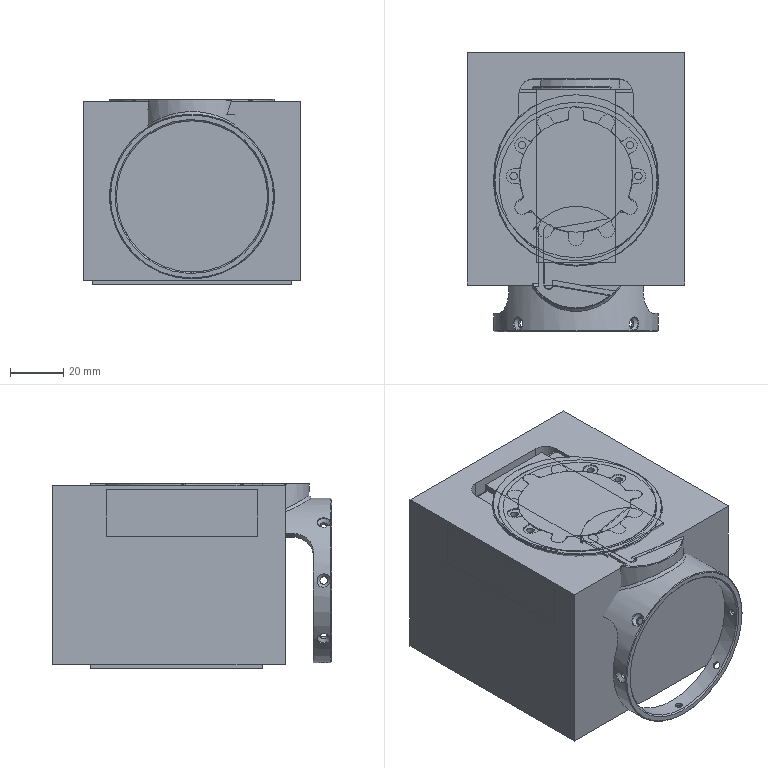NC program | NX | posted with a generic post | part box 82 x 105.2 x 70 mm
Lines 22992 to 23469 of 123648:
(单向轮廓精光_3_COPY_1_COPY_COPY_COPY_COPY , TOOL : 光刀D4)
N45862 T07 M6
N45864 G53
N45866 G18 G0 G90 X15.218 Z-47.555 S12000 M3
N45868 G43 Y73.855 H7
N45870 Y28.155
N45872 G41 G94 G1 Z-42.355 F700. D7
N45874 Z-40.63
N45876 G2 X13.549 Z-38.641 R2.02
N45878 G1 X-8.153 Z-34.814
N45880 G2 X-9.46 Z-35.024 R2.02
N45882 G1 X-9.622 Z-35.111
N45884 X-9.78 Z-35.206
N45886 Z-20.749
N45888 G2 X-9.573 Z-20.877 R2.02
N45890 G1 X-9.407 Z-20.966
N45892 G2 X-8.1 Z-21.176 R2.02
N45894 G1 X13.298 Z-17.403
N45896 G2 X14.29 Z-16.923 R2.02
N45898 G1 X14.407 Z-16.819
N45900 G2 X14.783 Z-16.371 R2.02
N45902 G1 X14.917 Z-16.153
N45904 G2 X15.218 Z-15.092 R2.02
N45906 G1 Z-13.645
N45908 Z-8.645
N45910 G40
N45912 Z-8.445
N45914 G0 Y73.855
N45916 X15.198 Z-47.555
N45918 Y28.155
N45920 G41 G1 Z-42.355
N45922 Z-40.63
N45924 G2 X13.545 Z-38.661 R2.
N45926 G1 X-8.157 Z-34.834
N45928 G2 X-9.451 Z-35.042 R2.
N45930 G1 X-9.613 Z-35.129
N45932 G2 X-9.8 Z-35.243 R2.
N45934 G1 Z-20.71
N45936 G2 X-9.563 Z-20.86 R2.
N45938 G1 X-9.398 Z-20.949
N45940 G2 X-8.104 Z-21.157 R2.
N45942 G1 X13.294 Z-17.384
N45944 G2 X14.277 Z-16.908 R2.
N45946 G1 X14.393 Z-16.804
N45948 G2 X14.766 Z-16.36 R2.
N45950 G1 X14.9 Z-16.142
N45952 G2 X15.198 Z-15.092 R2.
N45954 G1 Z-13.645
N45956 Z-8.645
N45958 G40
N45960 Z-8.445
N45962 G0 Y73.855
(单向轮廓精光_3_COPY_1_COPY_COPY_COPY , TOOL : 光刀D4)
N45964 X15.417 Z-37.258
N45966 Y73.84
N45968 Y33.14
N45970 G41 G1 X14.878 Z-40.311
N45972 G3 X14.531 Z-40.554 R0.3
N45974 G1 X-9.437 Z-36.328
N45976 G3 X-9.68 Z-35.98 R0.3
N45978 G1 X-9.176 Z-33.124
N45980 G40
N45982 X-9.142 Z-32.927
N45984 X15.417 Z-37.258
N45986 G41 X14.875 Z-40.33
N45988 G3 X14.527 Z-40.574 R0.3
N45990 G1 X-9.44 Z-36.348
N45992 G3 X-9.684 Z-36. R0.3
N45994 G1 X-9.176 Z-33.124
N45996 G40
N45998 X-9.142 Z-32.927
N46000 G0 Y73.84
N46002 Z-23.073
N46004 Y33.14
N46006 G41 G1 X-9.68 Z-20.02
N46008 G3 X-9.437 Z-19.672 R0.3
N46010 G1 X14.531 Z-15.446
N46012 G3 X14.878 Z-15.689 R0.3
N46014 G1 X15.382 Z-18.545
N46016 G40
N46018 X15.417 Z-18.742
N46020 X-9.142 Z-23.073
N46022 G41 X-9.683 Z-20.
N46024 G3 X-9.44 Z-19.652 R0.3
N46026 G1 X14.527 Z-15.426
N46028 G3 X14.875 Z-15.67 R0.3
N46030 G1 X15.382 Z-18.545
N46032 G40
N46034 X15.417 Z-18.742
N46036 G0 Y73.84
(底壁铣选底 , TOOL : 光刀D4)
N46038 Y77.5 S8000
N46040 X21.88 Z-30.292
N46042 Y29.15
N46044 G1 Y28.15 F1200.
N46046 X21.363 Z-30.874
N46048 G3 X20.798 Z-30.907 R0.4
N46050 G2 X15.681 Z-28.426 R10.4
N46052 G1 X13.264 Z-28.
N46054 X10.783
N46056 X13.264
N46058 X15.681 Z-27.574
N46060 G2 X20.798 Z-25.093 R10.4
N46062 X20.174 Z-22.168 R21.
N46064 G1 X19.061 Z-23.158
N46066 G3 X15.23 Z-25.013 R7.8
N46068 G1 X-1.708 Z-28.
N46070 X15.23 Z-30.987
N46072 G3 X19.061 Z-32.842 R7.8
N46074 G1 X20.174 Z-33.832
N46076 G3 X19.116 Z-36.693 R21.
N46078 G1 X18.677 Z-35.98
N46080 X17.333 Z-34.784
N46082 G2 X14.779 Z-33.547 R5.2
N46084 G1 X-4.55 Z-30.139
N46086 Z-25.861
N46088 X14.779 Z-22.453
N46090 G2 X17.333 Z-21.216 R5.2
N46092 G1 X18.677 Z-20.02
N46094 X19.116 Z-19.307
N46096 G2 X17.662 Z-16.64 R21.
N46098 G3 X17.461 Z-17.039 R2.6
N46100 G1 X16.664 Z-18.331
N46102 X15.604 Z-19.274
N46104 G3 X14.327 Z-19.892 R2.6
N46106 G1 X-7.15 Z-23.679
N46108 Z-32.321
N46110 X14.327 Z-36.108
N46112 G3 X15.604 Z-36.726 R2.6
N46114 G1 X16.664 Z-37.669
N46116 X17.461 Z-38.961
N46118 G3 X17.662 Z-39.36 R2.6
N46120 X15.401 Z-42.276 R21.
N46122 X15.248 Z-42.439 R21.
N46124 G1 Z-40.326
N46126 X14.651 Z-39.358
N46128 X13.876 Z-38.668
N46130 X-8.848 Z-34.661
N46132 X-9.636 Z-35.085
N46134 X-9.75 Z-35.151
N46136 Z-20.806
N46138 X-9.675 Z-20.857
N46140 X-9.587 Z-20.904
N46142 X-8.795 Z-21.329
N46144 X13.876 Z-17.332
N46146 X14.651 Z-16.642
N46148 X15.248 Z-15.674
N46150 Z-13.56
N46152 G3 X15.648 Z-13.16 R0.4
N46154 G1 X16.248
N46156 Y29.15
N46158 G0 Y77.5
N46160 M5
(单向轮廓精光_4 , TOOL : D10加长刀)
N46162 T10 M6
N46164 G53
N46166 G17 G0 G90 X25.02 Y43.85 S4500 M3
N46168 G43 Z40. H10
N46170 Z-56.5
N46172 G94 G1 Z-59.5 F700.
N46174 G41 Y35.65 D10
N46176 Y23.889
N46178 G3 X25.593 Y22.496 R1.98
N46180 G2 X-25.593 Y22.496 R-36.02
N46182 G3 X-25.02 Y23.889 R1.98
N46184 G1 Y35.65
N46186 Y43.65
N46188 G40
N46190 Y43.85
N46192 Z-56.5
N46194 G0 Z40.
N46196 X25.
N46198 Z-56.5
N46200 G1 Z-59.5
N46202 G41 Y35.65
N46204 Y23.889
N46206 G3 X25.579 Y22.482 R2.
N46208 G2 X-25.579 Y22.482 R-36.
N46210 G3 X-25. Y23.889 R2.
N46212 G1 Y35.65
N46214 Y43.65
N46216 G40
N46218 Y43.85
N46220 Z-56.5
N46222 G0 Z40.
N46224 X25.
N46226 Z-56.5
N46228 G1 Z-59.5
N46230 G41 Y35.65
N46232 Y23.889
N46234 G3 X25.579 Y22.482 R2.
N46236 G2 X-25.579 Y22.482 R-36.
N46238 G3 X-25. Y23.889 R2.
N46240 G1 Y35.65
N46242 Y43.65
N46244 G40
N46246 Y43.85
N46248 Z-56.5
N46250 G0 Z40.
N46252 X25.
N46254 Z-56.5
N46256 G1 Z-59.5
N46258 G41 Y35.65
N46260 Y23.889
N46262 G3 X25.579 Y22.482 R2.
N46264 G2 X-25.579 Y22.482 R-36.
N46266 G3 X-25. Y23.889 R2.
N46268 G1 Y35.65
N46270 Y43.65
N46272 G40
N46274 Y43.85
N46276 Z-56.5
N46278 G0 Z40.
N46280 M5
(单向轮廓精光_5 , TOOL : 光刀D8)
N46282 T08 M6
N46284 G53
N46286 G18 G0 G90 X1. Z-30.205 S8000 M3
N46288 G43 Y73.85 H8
N46290 Y23.15
N46292 G94 G1 Y20.15 F1200.
N46294 G41 Z-32.005 D8
N46296 G3 X0. Z-33.005 R1.
N46298 X-5.005 Z-28. R5.005
N46300 X0. Z-33.005 R-5.005
N46302 X-0.499 Z-32.98 R5.005
N46304 X-1.394 Z-31.885 R1.
N46306 G40
N46308 G1 X-1.375 Z-31.686
N46310 X1. Z-31.825
N46312 G41 Z-32.025
N46314 G3 X0. Z-33.025 R1.
N46316 X-5.025 Z-28. R5.025
N46318 X0. Z-33.025 R-5.025
N46320 X-0.499 Z-33. R5.025
N46322 X-1.395 Z-31.906 R1.
N46324 G1 X-1.236 Z-30.316
N46326 G40
N46328 X-1.216 Z-30.117
N46330 Y23.15
N46332 G0 Y73.85
N46334 M5
(VARIABLE_CONTOUR_COPY_2 , TOOL : 45度燕尾刀D6)
N46336 T09 M6
N46338 G53
N46340 G18 G0 G90 X19.636 Z-38.568 S8000 M3
N46342 G43 Y43.85 H9
N46344 Y33.133
N46346 G94 G1 X13.727 Z-37.526 F3000.
N46348 X-8.271 Z-33.648
N46350 Y33.047 Z-33.679
N46352 X13.727 Z-37.558
N46354 Y32.939 Z-37.597
N46356 X-8.271 Z-33.719
N46358 Y32.852 Z-33.75
N46360 X13.727 Z-37.629
N46362 Y32.744 Z-37.669
N46364 X-8.271 Z-33.79
N46366 Y32.658 Z-33.821
N46368 X13.727 Z-37.7
N46370 Y32.55 Z-37.74
N46372 X-8.271 Z-33.861
N46374 Y32.463 Z-33.892
N46376 X13.727 Z-37.771
N46378 Y32.355 Z-37.811
N46380 X-8.271 Z-33.932
N46382 Y32.269 Z-33.963
N46384 X13.727 Z-37.842
N46386 Y32.161 Z-37.882
N46388 X-8.271 Z-34.003
N46390 Y32.075 Z-34.034
N46392 X13.727 Z-37.913
N46394 Y31.967 Z-37.953
N46396 X-8.271 Z-34.074
N46398 Y31.88 Z-34.106
N46400 X13.727 Z-37.984
N46402 Y31.772 Z-38.024
N46404 X-8.271 Z-34.145
N46406 Y31.686 Z-34.177
N46408 X13.727 Z-38.055
N46410 Y31.578 Z-38.095
N46412 X-8.271 Z-34.216
N46414 Y31.491 Z-34.248
N46416 X13.727 Z-38.126
N46418 Y31.383 Z-38.166
N46420 X-8.271 Z-34.287
N46422 Y31.297 Z-34.319
N46424 X13.727 Z-38.198
N46426 Y31.189 Z-38.237
N46428 X-8.271 Z-34.358
N46430 Y31.103 Z-34.39
N46432 X13.727 Z-38.269
N46434 Y30.995 Z-38.308
N46436 X-8.271 Z-34.429
N46438 Y30.908 Z-34.461
N46440 X13.727 Z-38.34
N46442 Y30.8 Z-38.379
N46444 X-8.271 Z-34.5
N46446 Y30.714 Z-34.532
N46448 X13.727 Z-38.411
N46450 Y30.606 Z-38.45
N46452 X-8.271 Z-34.571
N46454 Y30.519 Z-34.603
N46456 X13.727 Z-38.482
N46458 Y30.411 Z-38.521
N46460 X-8.271 Z-34.642
N46462 Y30.325 Z-34.674
N46464 X13.727 Z-38.553
N46466 Y30.217 Z-38.592
N46468 X-8.271 Z-34.714
N46470 Y30.131 Z-34.745
N46472 X13.727 Z-38.624
N46474 Y30.023 Z-38.663
N46476 X-8.271 Z-34.785
N46478 Y29.936 Z-34.816
N46480 X13.727 Z-38.695
N46482 Y29.828 Z-38.734
N46484 X-8.271 Z-34.856
N46486 Y29.742 Z-34.887
N46488 X13.727 Z-38.766
N46490 Y29.634 Z-38.806
N46492 X-8.271 Z-34.927
N46494 Y29.547 Z-34.958
N46496 X13.727 Z-38.837
N46498 Y29.439 Z-38.877
N46500 X-8.271 Z-34.998
N46502 Y29.353 Z-35.029
N46504 X13.727 Z-38.908
N46506 Y29.245 Z-38.948
N46508 X-8.271 Z-35.069
N46510 Y29.159 Z-35.1
N46512 X13.727 Z-38.979
N46514 Y29.051 Z-39.019
N46516 X-8.271 Z-35.14
N46518 Y28.964 Z-35.171
N46520 X13.727 Z-39.05
N46522 Y28.856 Z-39.09
N46524 X-8.271 Z-35.211
N46526 Y28.77 Z-35.243
N46528 X13.727 Z-39.121
N46530 Y28.662 Z-39.161
N46532 X-8.271 Z-35.282
N46534 Y28.575 Z-35.314
N46536 X13.727 Z-39.192
N46538 Y28.467 Z-39.232
N46540 X-8.271 Z-35.353
N46542 Y28.381 Z-35.385
N46544 X13.727 Z-39.264
N46546 Y28.273 Z-39.303
N46548 X-8.271 Z-35.424
N46550 Y28.208 Z-35.448
N46552 X13.727 Z-39.327
N46554 X19.636 Z-40.369
N46556 G0 Y43.85
(VARIABLE_CONTOUR_COPY_2_COPY , TOOL : 45度燕尾刀D6)
N46558 Z-17.432
N46560 Y33.133
N46562 G1 X13.727 Z-18.474
N46564 X-8.271 Z-22.352
N46566 Y33.025 Z-22.313
N46568 X13.727 Z-18.434
N46570 Y32.939 Z-18.403
N46572 X-8.271 Z-22.281
N46574 Y32.831 Z-22.242
N46576 X13.727 Z-18.363
N46578 Y32.744 Z-18.331
N46580 X-8.271 Z-22.21
N46582 Y32.636 Z-22.171
N46584 X13.727 Z-18.292
N46586 Y32.55 Z-18.26
N46588 X-8.271 Z-22.139
N46590 Y32.442 Z-22.1
N46592 X13.727 Z-18.221
N46594 Y32.355 Z-18.189
N46596 X-8.271 Z-22.068
N46598 Y32.247 Z-22.029
N46600 X13.727 Z-18.15
N46602 Y32.161 Z-18.118
N46604 X-8.271 Z-21.997
N46606 Y32.053 Z-21.958
N46608 X13.727 Z-18.079
N46610 Y31.967 Z-18.047
N46612 X-8.271 Z-21.926
N46614 Y31.859 Z-21.887
N46616 X13.727 Z-18.008
N46618 Y31.772 Z-17.976
N46620 X-8.271 Z-21.855
N46622 Y31.664 Z-21.816
N46624 X13.727 Z-17.937
N46626 Y31.578 Z-17.905
N46628 X-8.271 Z-21.784
N46630 Y31.47 Z-21.744
N46632 X13.727 Z-17.866
N46634 Y31.383 Z-17.834
N46636 X-8.271 Z-21.713
N46638 Y31.275 Z-21.673
N46640 X13.727 Z-17.795
N46642 Y31.189 Z-17.763
N46644 X-8.271 Z-21.642
N46646 Y31.081 Z-21.602
N46648 X13.727 Z-17.723
N46650 Y30.995 Z-17.692
N46652 X-8.271 Z-21.571
N46654 Y30.887 Z-21.531
N46656 X13.727 Z-17.652
N46658 Y30.8 Z-17.621
N46660 X-8.271 Z-21.5
N46662 Y30.692 Z-21.46
N46664 X13.727 Z-17.581
N46666 Y30.606 Z-17.55
N46668 X-8.271 Z-21.429
N46670 Y30.498 Z-21.389
N46672 X13.727 Z-17.51
N46674 Y30.411 Z-17.479
N46676 X-8.271 Z-21.358
N46678 Y30.303 Z-21.318
N46680 X13.727 Z-17.439
N46682 Y30.217 Z-17.408
N46684 X-8.271 Z-21.286
N46686 Y30.109 Z-21.247
N46688 X13.727 Z-17.368
N46690 Y30.023 Z-17.337
N46692 X-8.271 Z-21.215
N46694 Y29.915 Z-21.176
N46696 X13.727 Z-17.297
N46698 Y29.828 Z-17.266
N46700 X-8.271 Z-21.144
N46702 Y29.72 Z-21.105
N46704 X13.727 Z-17.226
N46706 Y29.634 Z-17.194
N46708 X-8.271 Z-21.073
N46710 Y29.526 Z-21.034
N46712 X13.727 Z-17.155
N46714 Y29.439 Z-17.123
N46716 X-8.271 Z-21.002
N46718 Y29.331 Z-20.963
N46720 X13.727 Z-17.084
N46722 Y29.245 Z-17.052
N46724 X-8.271 Z-20.931
N46726 Y29.137 Z-20.892
N46728 X13.727 Z-17.013
N46730 Y29.051 Z-16.981
N46732 X-8.271 Z-20.86
N46734 Y28.943 Z-20.821
N46736 X13.727 Z-16.942
N46738 Y28.856 Z-16.91
N46740 X-8.271 Z-20.789
N46742 Y28.748 Z-20.75
N46744 X13.727 Z-16.871
N46746 Y28.662 Z-16.839
N46748 X-8.271 Z-20.718
N46750 Y28.554 Z-20.678
N46752 X13.727 Z-16.8
N46754 Y28.467 Z-16.768
N46756 X-8.271 Z-20.647
N46758 Y28.359 Z-20.607
N46760 X13.727 Z-16.729
N46762 Y28.273 Z-16.697
N46764 X-8.271 Z-20.576
N46766 Y28.208 Z-20.552
N46768 X13.727 Z-16.673
N46770 X19.636 Z-15.631
N46772 G0 Y43.85
N46774 M5